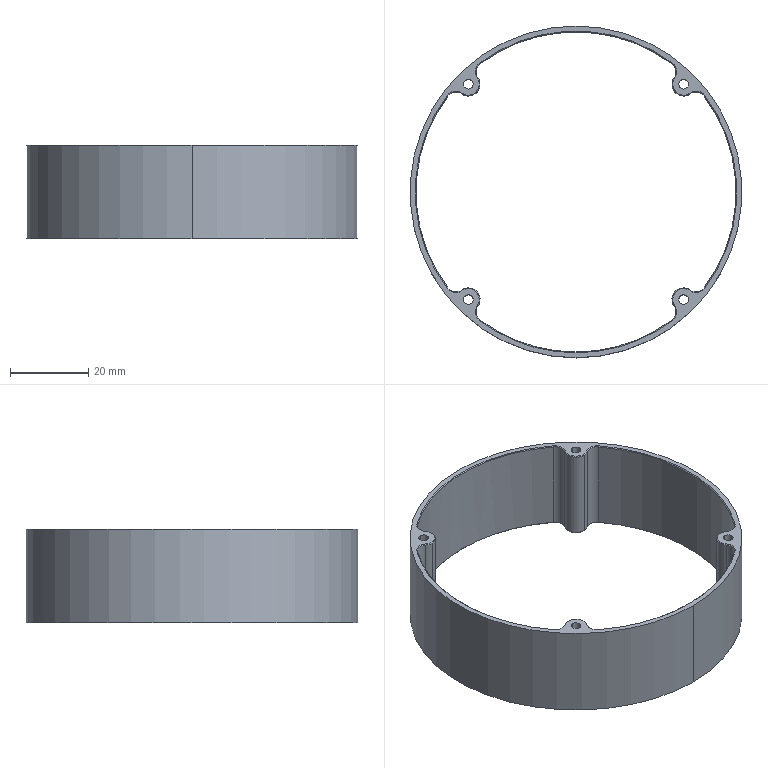NC program | NX | posted with a generic post | part box 85 x 85 x 24 mm
Lines 138 to 991 of 6793:
(PLANAR_MILL , TOOL : D10)
N250 T15 M6
N252 G54
N254 G17 G0 G90 X-2.703 Y-7.279 S9500 M3
N256 G43 Z30. H15
N258 Z1.
N260 G94 G1 X-2.578 Y-7.426 Z0.99 F1000.
N262 X-1.45 Y-8.911 Z0.892
N264 X-0.41 Y-10.46 Z0.794
N266 X0. Y-11.148 Z0.752
N268 X0.41 Y-10.46 Z0.71
N270 X1.45 Y-8.911 Z0.613
N272 X2.578 Y-7.426 Z0.515
N274 X3.79 Y-6.008 Z0.417
N276 X4.873 Y-4.873 Z0.335
N278 X6.008 Y-3.79 Z0.253
N280 X7.426 Y-2.578 Z0.155
N282 X8.911 Y-1.45 Z0.057
N284 X10.46 Y-0.41 Z-0.041
N286 X11.148 Y0. Z-0.083
N288 X10.46 Y0.41 Z-0.125
N290 X8.911 Y1.45 Z-0.222
N292 X7.426 Y2.578 Z-0.32
N294 X6.008 Y3.79 Z-0.418
N296 X4.879 Y4.879 Z-0.5
N298 X0.636 Y0.636
N300 G2 X0. Y1.288 R38.1 F2200.
N302 X-1.288 Y0. R38.1
N304 X0. Y-1.288 R38.1
N306 X1.288 Y0. R38.1
N308 X0.636 Y0.636 R38.1
N310 G1 X4.879 Y4.879
N312 G2 X0. Y11.148 R32.1
N314 X-11.148 Y0. R32.1
N316 X0. Y-11.148 R32.1
N318 X11.148 Y0. R32.1
N320 X4.879 Y4.879 R32.1
N322 G1 X9.122 Y9.122
N324 G2 X3.476 Y17.559 R26.1
N326 G3 X-3.476 Y17.559 R17.9
N328 G2 X-17.559 Y3.476 R26.1
N330 G3 X-17.559 Y-3.476 R17.9
N332 G2 X-3.476 Y-17.559 R26.1
N334 G3 X3.476 Y-17.559 R17.9
N336 G2 X17.559 Y-3.476 R26.1
N338 G3 X17.559 Y3.476 R17.9
N340 G2 X9.122 Y9.122 R26.1
N342 G1 X13.364 Y13.364
N344 G2 X8.136 Y22.472 R20.1
N346 G3 X-8.136 Y22.472 R23.9
N348 G2 X-22.472 Y8.136 R20.1
N350 G3 X-22.472 Y-8.136 R23.9
N352 G2 X-8.136 Y-22.472 R20.1
N354 G3 X8.136 Y-22.472 R23.9
N356 G2 X22.472 Y-8.136 R20.1
N358 G3 X22.472 Y8.136 R23.9
N360 G2 X13.364 Y13.364 R20.1
N362 G1 X17.607 Y17.607
N364 G2 X13.506 Y26.676 R14.1
N366 G3 X-13.506 Y26.676 R29.9
N368 G2 X-26.676 Y13.506 R14.1
N370 G3 X-26.676 Y-13.506 R29.9
N372 G2 X-13.506 Y-26.676 R14.1
N374 G3 X13.506 Y-26.676 R29.9
N376 G2 X26.676 Y-13.506 R14.1
N378 G3 X26.676 Y13.506 R29.9
N380 G2 X17.607 Y17.607 R14.1
N382 G1 X21.85 Y21.85
N384 G2 X19.826 Y29.929 R8.1
N386 G3 X-19.826 Y29.929 R35.9
N388 G2 X-29.929 Y19.826 R8.1
N390 G3 X-29.929 Y-19.826 R35.9
N392 G2 X-19.826 Y-29.929 R8.1
N394 G3 X19.826 Y-29.929 R35.9
N396 G2 X29.929 Y-19.826 R8.1
N398 G3 X29.929 Y19.826 R35.9
N400 G2 X21.85 Y21.85 R8.1
N402 G1 Z0.5
N404 G0 X-2.703 Y-7.279
N406 G1 X-2.578 Y-7.426 Z0.49 F1000.
N408 X-1.45 Y-8.911 Z0.392
N410 X-0.41 Y-10.46 Z0.294
N412 X0. Y-11.148 Z0.252
N414 X0.41 Y-10.46 Z0.21
N416 X1.45 Y-8.911 Z0.113
N418 X2.578 Y-7.426 Z0.015
N420 X3.79 Y-6.008 Z-0.083
N422 X4.873 Y-4.873 Z-0.165
N424 X6.008 Y-3.79 Z-0.247
N426 X7.426 Y-2.578 Z-0.345
N428 X8.911 Y-1.45 Z-0.443
N430 X10.46 Y-0.41 Z-0.541
N432 X11.148 Y0. Z-0.583
N434 X10.46 Y0.41 Z-0.625
N436 X8.911 Y1.45 Z-0.722
N438 X7.426 Y2.578 Z-0.82
N440 X6.008 Y3.79 Z-0.918
N442 X4.879 Y4.879 Z-1.
N444 X0.636 Y0.636
N446 G2 X0. Y1.288 R38.1 F2200.
N448 X-1.288 Y0. R38.1
N450 X0. Y-1.288 R38.1
N452 X1.288 Y0. R38.1
N454 X0.636 Y0.636 R38.1
N456 G1 X4.879 Y4.879
N458 G2 X0. Y11.148 R32.1
N460 X-11.148 Y0. R32.1
N462 X0. Y-11.148 R32.1
N464 X11.148 Y0. R32.1
N466 X4.879 Y4.879 R32.1
N468 G1 X9.122 Y9.122
N470 G2 X3.476 Y17.559 R26.1
N472 G3 X-3.476 Y17.559 R17.9
N474 G2 X-17.559 Y3.476 R26.1
N476 G3 X-17.559 Y-3.476 R17.9
N478 G2 X-3.476 Y-17.559 R26.1
N480 G3 X3.476 Y-17.559 R17.9
N482 G2 X17.559 Y-3.476 R26.1
N484 G3 X17.559 Y3.476 R17.9
N486 G2 X9.122 Y9.122 R26.1
N488 G1 X13.364 Y13.364
N490 G2 X8.136 Y22.472 R20.1
N492 G3 X-8.136 Y22.472 R23.9
N494 G2 X-22.472 Y8.136 R20.1
N496 G3 X-22.472 Y-8.136 R23.9
N498 G2 X-8.136 Y-22.472 R20.1
N500 G3 X8.136 Y-22.472 R23.9
N502 G2 X22.472 Y-8.136 R20.1
N504 G3 X22.472 Y8.136 R23.9
N506 G2 X13.364 Y13.364 R20.1
N508 G1 X17.607 Y17.607
N510 G2 X13.506 Y26.676 R14.1
N512 G3 X-13.506 Y26.676 R29.9
N514 G2 X-26.676 Y13.506 R14.1
N516 G3 X-26.676 Y-13.506 R29.9
N518 G2 X-13.506 Y-26.676 R14.1
N520 G3 X13.506 Y-26.676 R29.9
N522 G2 X26.676 Y-13.506 R14.1
N524 G3 X26.676 Y13.506 R29.9
N526 G2 X17.607 Y17.607 R14.1
N528 G1 X21.85 Y21.85
N530 G2 X19.826 Y29.929 R8.1
N532 G3 X-19.826 Y29.929 R35.9
N534 G2 X-29.929 Y19.826 R8.1
N536 G3 X-29.929 Y-19.826 R35.9
N538 G2 X-19.826 Y-29.929 R8.1
N540 G3 X19.826 Y-29.929 R35.9
N542 G2 X29.929 Y-19.826 R8.1
N544 G3 X29.929 Y19.826 R35.9
N546 G2 X21.85 Y21.85 R8.1
N548 G1 Z0.
N550 G0 X-2.703 Y-7.279
N552 G1 X-2.578 Y-7.426 Z-0.01 F1000.
N554 X-1.45 Y-8.911 Z-0.108
N556 X-0.41 Y-10.46 Z-0.206
N558 X0. Y-11.148 Z-0.248
N560 X0.41 Y-10.46 Z-0.29
N562 X1.45 Y-8.911 Z-0.387
N564 X2.578 Y-7.426 Z-0.485
N566 X3.79 Y-6.008 Z-0.583
N568 X4.873 Y-4.873 Z-0.665
N570 X6.008 Y-3.79 Z-0.747
N572 X7.426 Y-2.578 Z-0.845
N574 X8.911 Y-1.45 Z-0.943
N576 X10.46 Y-0.41 Z-1.041
N578 X11.148 Y0. Z-1.083
N580 X10.46 Y0.41 Z-1.125
N582 X8.911 Y1.45 Z-1.222
N584 X7.426 Y2.578 Z-1.32
N586 X6.008 Y3.79 Z-1.418
N588 X4.879 Y4.879 Z-1.5
N590 X0.636 Y0.636
N592 G2 X0. Y1.288 R38.1 F2200.
N594 X-1.288 Y0. R38.1
N596 X0. Y-1.288 R38.1
N598 X1.288 Y0. R38.1
N600 X0.636 Y0.636 R38.1
N602 G1 X4.879 Y4.879
N604 G2 X0. Y11.148 R32.1
N606 X-11.148 Y0. R32.1
N608 X0. Y-11.148 R32.1
N610 X11.148 Y0. R32.1
N612 X4.879 Y4.879 R32.1
N614 G1 X9.122 Y9.122
N616 G2 X3.476 Y17.559 R26.1
N618 G3 X-3.476 Y17.559 R17.9
N620 G2 X-17.559 Y3.476 R26.1
N622 G3 X-17.559 Y-3.476 R17.9
N624 G2 X-3.476 Y-17.559 R26.1
N626 G3 X3.476 Y-17.559 R17.9
N628 G2 X17.559 Y-3.476 R26.1
N630 G3 X17.559 Y3.476 R17.9
N632 G2 X9.122 Y9.122 R26.1
N634 G1 X13.364 Y13.364
N636 G2 X8.136 Y22.472 R20.1
N638 G3 X-8.136 Y22.472 R23.9
N640 G2 X-22.472 Y8.136 R20.1
N642 G3 X-22.472 Y-8.136 R23.9
N644 G2 X-8.136 Y-22.472 R20.1
N646 G3 X8.136 Y-22.472 R23.9
N648 G2 X22.472 Y-8.136 R20.1
N650 G3 X22.472 Y8.136 R23.9
N652 G2 X13.364 Y13.364 R20.1
N654 G1 X17.607 Y17.607
N656 G2 X13.506 Y26.676 R14.1
N658 G3 X-13.506 Y26.676 R29.9
N660 G2 X-26.676 Y13.506 R14.1
N662 G3 X-26.676 Y-13.506 R29.9
N664 G2 X-13.506 Y-26.676 R14.1
N666 G3 X13.506 Y-26.676 R29.9
N668 G2 X26.676 Y-13.506 R14.1
N670 G3 X26.676 Y13.506 R29.9
N672 G2 X17.607 Y17.607 R14.1
N674 G1 X21.85 Y21.85
N676 G2 X19.826 Y29.929 R8.1
N678 G3 X-19.826 Y29.929 R35.9
N680 G2 X-29.929 Y19.826 R8.1
N682 G3 X-29.929 Y-19.826 R35.9
N684 G2 X-19.826 Y-29.929 R8.1
N686 G3 X19.826 Y-29.929 R35.9
N688 G2 X29.929 Y-19.826 R8.1
N690 G3 X29.929 Y19.826 R35.9
N692 G2 X21.85 Y21.85 R8.1
N694 G1 Z-0.5
N696 G0 X-2.703 Y-7.279
N698 G1 X-2.578 Y-7.426 Z-0.51 F1000.
N700 X-1.45 Y-8.911 Z-0.608
N702 X-0.41 Y-10.46 Z-0.706
N704 X0. Y-11.148 Z-0.748
N706 X0.41 Y-10.46 Z-0.79
N708 X1.45 Y-8.911 Z-0.887
N710 X2.578 Y-7.426 Z-0.985
N712 X3.79 Y-6.008 Z-1.083
N714 X4.873 Y-4.873 Z-1.165
N716 X6.008 Y-3.79 Z-1.247
N718 X7.426 Y-2.578 Z-1.345
N720 X8.911 Y-1.45 Z-1.443
N722 X10.46 Y-0.41 Z-1.541
N724 X11.148 Y0. Z-1.583
N726 X10.46 Y0.41 Z-1.625
N728 X8.911 Y1.45 Z-1.722
N730 X7.426 Y2.578 Z-1.82
N732 X6.008 Y3.79 Z-1.918
N734 X4.879 Y4.879 Z-2.
N736 X0.636 Y0.636
N738 G2 X0. Y1.288 R38.1 F2200.
N740 X-1.288 Y0. R38.1
N742 X0. Y-1.288 R38.1
N744 X1.288 Y0. R38.1
N746 X0.636 Y0.636 R38.1
N748 G1 X4.879 Y4.879
N750 G2 X0. Y11.148 R32.1
N752 X-11.148 Y0. R32.1
N754 X0. Y-11.148 R32.1
N756 X11.148 Y0. R32.1
N758 X4.879 Y4.879 R32.1
N760 G1 X9.122 Y9.122
N762 G2 X3.476 Y17.559 R26.1
N764 G3 X-3.476 Y17.559 R17.9
N766 G2 X-17.559 Y3.476 R26.1
N768 G3 X-17.559 Y-3.476 R17.9
N770 G2 X-3.476 Y-17.559 R26.1
N772 G3 X3.476 Y-17.559 R17.9
N774 G2 X17.559 Y-3.476 R26.1
N776 G3 X17.559 Y3.476 R17.9
N778 G2 X9.122 Y9.122 R26.1
N780 G1 X13.364 Y13.364
N782 G2 X8.136 Y22.472 R20.1
N784 G3 X-8.136 Y22.472 R23.9
N786 G2 X-22.472 Y8.136 R20.1
N788 G3 X-22.472 Y-8.136 R23.9
N790 G2 X-8.136 Y-22.472 R20.1
N792 G3 X8.136 Y-22.472 R23.9
N794 G2 X22.472 Y-8.136 R20.1
N796 G3 X22.472 Y8.136 R23.9
N798 G2 X13.364 Y13.364 R20.1
N800 G1 X17.607 Y17.607
N802 G2 X13.506 Y26.676 R14.1
N804 G3 X-13.506 Y26.676 R29.9
N806 G2 X-26.676 Y13.506 R14.1
N808 G3 X-26.676 Y-13.506 R29.9
N810 G2 X-13.506 Y-26.676 R14.1
N812 G3 X13.506 Y-26.676 R29.9
N814 G2 X26.676 Y-13.506 R14.1
N816 G3 X26.676 Y13.506 R29.9
N818 G2 X17.607 Y17.607 R14.1
N820 G1 X21.85 Y21.85
N822 G2 X19.826 Y29.929 R8.1
N824 G3 X-19.826 Y29.929 R35.9
N826 G2 X-29.929 Y19.826 R8.1
N828 G3 X-29.929 Y-19.826 R35.9
N830 G2 X-19.826 Y-29.929 R8.1
N832 G3 X19.826 Y-29.929 R35.9
N834 G2 X29.929 Y-19.826 R8.1
N836 G3 X29.929 Y19.826 R35.9
N838 G2 X21.85 Y21.85 R8.1
N840 G1 Z-1.
N842 G0 X-2.703 Y-7.279
N844 G1 X-2.578 Y-7.426 Z-1.01 F1000.
N846 X-1.45 Y-8.911 Z-1.108
N848 X-0.41 Y-10.46 Z-1.206
N850 X0. Y-11.148 Z-1.248
N852 X0.41 Y-10.46 Z-1.29
N854 X1.45 Y-8.911 Z-1.387
N856 X2.578 Y-7.426 Z-1.485
N858 X3.79 Y-6.008 Z-1.583
N860 X4.873 Y-4.873 Z-1.665
N862 X6.008 Y-3.79 Z-1.747
N864 X7.426 Y-2.578 Z-1.845
N866 X8.911 Y-1.45 Z-1.943
N868 X10.46 Y-0.41 Z-2.041
N870 X11.148 Y0. Z-2.083
N872 X10.46 Y0.41 Z-2.125
N874 X8.911 Y1.45 Z-2.222
N876 X7.426 Y2.578 Z-2.32
N878 X6.008 Y3.79 Z-2.418
N880 X4.879 Y4.879 Z-2.5
N882 X0.636 Y0.636
N884 G2 X0. Y1.288 R38.1 F2200.
N886 X-1.288 Y0. R38.1
N888 X0. Y-1.288 R38.1
N890 X1.288 Y0. R38.1
N892 X0.636 Y0.636 R38.1
N894 G1 X4.879 Y4.879
N896 G2 X0. Y11.148 R32.1
N898 X-11.148 Y0. R32.1
N900 X0. Y-11.148 R32.1
N902 X11.148 Y0. R32.1
N904 X4.879 Y4.879 R32.1
N906 G1 X9.122 Y9.122
N908 G2 X3.476 Y17.559 R26.1
N910 G3 X-3.476 Y17.559 R17.9
N912 G2 X-17.559 Y3.476 R26.1
N914 G3 X-17.559 Y-3.476 R17.9
N916 G2 X-3.476 Y-17.559 R26.1
N918 G3 X3.476 Y-17.559 R17.9
N920 G2 X17.559 Y-3.476 R26.1
N922 G3 X17.559 Y3.476 R17.9
N924 G2 X9.122 Y9.122 R26.1
N926 G1 X13.364 Y13.364
N928 G2 X8.136 Y22.472 R20.1
N930 G3 X-8.136 Y22.472 R23.9
N932 G2 X-22.472 Y8.136 R20.1
N934 G3 X-22.472 Y-8.136 R23.9
N936 G2 X-8.136 Y-22.472 R20.1
N938 G3 X8.136 Y-22.472 R23.9
N940 G2 X22.472 Y-8.136 R20.1
N942 G3 X22.472 Y8.136 R23.9
N944 G2 X13.364 Y13.364 R20.1
N946 G1 X17.607 Y17.607
N948 G2 X13.506 Y26.676 R14.1
N950 G3 X-13.506 Y26.676 R29.9
N952 G2 X-26.676 Y13.506 R14.1
N954 G3 X-26.676 Y-13.506 R29.9
N956 G2 X-13.506 Y-26.676 R14.1
N958 G3 X13.506 Y-26.676 R29.9
N960 G2 X26.676 Y-13.506 R14.1
N962 G3 X26.676 Y13.506 R29.9
N964 G2 X17.607 Y17.607 R14.1
N966 G1 X21.85 Y21.85
N968 G2 X19.826 Y29.929 R8.1
N970 G3 X-19.826 Y29.929 R35.9
N972 G2 X-29.929 Y19.826 R8.1
N974 G3 X-29.929 Y-19.826 R35.9
N976 G2 X-19.826 Y-29.929 R8.1
N978 G3 X19.826 Y-29.929 R35.9
N980 G2 X29.929 Y-19.826 R8.1
N982 G3 X29.929 Y19.826 R35.9
N984 G2 X21.85 Y21.85 R8.1
N986 G1 Z-1.5
N988 G0 X-2.703 Y-7.279
N990 G1 X-2.578 Y-7.426 Z-1.51 F1000.
N992 X-1.45 Y-8.911 Z-1.608
N994 X-0.41 Y-10.46 Z-1.706
N996 X0. Y-11.148 Z-1.748
N998 X0.41 Y-10.46 Z-1.79
N1000 X1.45 Y-8.911 Z-1.887
N1002 X2.578 Y-7.426 Z-1.985
N1004 X3.79 Y-6.008 Z-2.083
N1006 X4.873 Y-4.873 Z-2.165
N1008 X6.008 Y-3.79 Z-2.247
N1010 X7.426 Y-2.578 Z-2.345
N1012 X8.911 Y-1.45 Z-2.443
N1014 X10.46 Y-0.41 Z-2.541
N1016 X11.148 Y0. Z-2.583
N1018 X10.46 Y0.41 Z-2.625
N1020 X8.911 Y1.45 Z-2.722
N1022 X7.426 Y2.578 Z-2.82
N1024 X6.008 Y3.79 Z-2.918
N1026 X4.879 Y4.879 Z-3.
N1028 X0.636 Y0.636
N1030 G2 X0. Y1.288 R38.1 F2200.
N1032 X-1.288 Y0. R38.1
N1034 X0. Y-1.288 R38.1
N1036 X1.288 Y0. R38.1
N1038 X0.636 Y0.636 R38.1
N1040 G1 X4.879 Y4.879
N1042 G2 X0. Y11.148 R32.1
N1044 X-11.148 Y0. R32.1
N1046 X0. Y-11.148 R32.1
N1048 X11.148 Y0. R32.1
N1050 X4.879 Y4.879 R32.1
N1052 G1 X9.122 Y9.122
N1054 G2 X3.476 Y17.559 R26.1
N1056 G3 X-3.476 Y17.559 R17.9
N1058 G2 X-17.559 Y3.476 R26.1
N1060 G3 X-17.559 Y-3.476 R17.9
N1062 G2 X-3.476 Y-17.559 R26.1
N1064 G3 X3.476 Y-17.559 R17.9
N1066 G2 X17.559 Y-3.476 R26.1
N1068 G3 X17.559 Y3.476 R17.9
N1070 G2 X9.122 Y9.122 R26.1
N1072 G1 X13.364 Y13.364
N1074 G2 X8.136 Y22.472 R20.1
N1076 G3 X-8.136 Y22.472 R23.9
N1078 G2 X-22.472 Y8.136 R20.1
N1080 G3 X-22.472 Y-8.136 R23.9
N1082 G2 X-8.136 Y-22.472 R20.1
N1084 G3 X8.136 Y-22.472 R23.9
N1086 G2 X22.472 Y-8.136 R20.1
N1088 G3 X22.472 Y8.136 R23.9
N1090 G2 X13.364 Y13.364 R20.1
N1092 G1 X17.607 Y17.607
N1094 G2 X13.506 Y26.676 R14.1
N1096 G3 X-13.506 Y26.676 R29.9
N1098 G2 X-26.676 Y13.506 R14.1
N1100 G3 X-26.676 Y-13.506 R29.9
N1102 G2 X-13.506 Y-26.676 R14.1
N1104 G3 X13.506 Y-26.676 R29.9
N1106 G2 X26.676 Y-13.506 R14.1
N1108 G3 X26.676 Y13.506 R29.9
N1110 G2 X17.607 Y17.607 R14.1
N1112 G1 X21.85 Y21.85
N1114 G2 X19.826 Y29.929 R8.1
N1116 G3 X-19.826 Y29.929 R35.9
N1118 G2 X-29.929 Y19.826 R8.1
N1120 G3 X-29.929 Y-19.826 R35.9
N1122 G2 X-19.826 Y-29.929 R8.1
N1124 G3 X19.826 Y-29.929 R35.9
N1126 G2 X29.929 Y-19.826 R8.1
N1128 G3 X29.929 Y19.826 R35.9
N1130 G2 X21.85 Y21.85 R8.1
N1132 G1 Z-2.
N1134 G0 X-2.703 Y-7.279
N1136 G1 X-2.578 Y-7.426 Z-2.01 F1000.
N1138 X-1.45 Y-8.911 Z-2.108
N1140 X-0.41 Y-10.46 Z-2.206
N1142 X0. Y-11.148 Z-2.248
N1144 X0.41 Y-10.46 Z-2.29
N1146 X1.45 Y-8.911 Z-2.387
N1148 X2.578 Y-7.426 Z-2.485
N1150 X3.79 Y-6.008 Z-2.583
N1152 X4.873 Y-4.873 Z-2.665
N1154 X6.008 Y-3.79 Z-2.747
N1156 X7.426 Y-2.578 Z-2.845
N1158 X8.911 Y-1.45 Z-2.943
N1160 X10.46 Y-0.41 Z-3.041
N1162 X11.148 Y0. Z-3.083
N1164 X10.46 Y0.41 Z-3.125
N1166 X8.911 Y1.45 Z-3.222
N1168 X7.426 Y2.578 Z-3.32
N1170 X6.008 Y3.79 Z-3.418
N1172 X4.879 Y4.879 Z-3.5
N1174 X0.636 Y0.636
N1176 G2 X0. Y1.288 R38.1 F2200.
N1178 X-1.288 Y0. R38.1
N1180 X0. Y-1.288 R38.1
N1182 X1.288 Y0. R38.1
N1184 X0.636 Y0.636 R38.1
N1186 G1 X4.879 Y4.879
N1188 G2 X0. Y11.148 R32.1
N1190 X-11.148 Y0. R32.1
N1192 X0. Y-11.148 R32.1
N1194 X11.148 Y0. R32.1
N1196 X4.879 Y4.879 R32.1
N1198 G1 X9.122 Y9.122
N1200 G2 X3.476 Y17.559 R26.1
N1202 G3 X-3.476 Y17.559 R17.9
N1204 G2 X-17.559 Y3.476 R26.1
N1206 G3 X-17.559 Y-3.476 R17.9
N1208 G2 X-3.476 Y-17.559 R26.1
N1210 G3 X3.476 Y-17.559 R17.9
N1212 G2 X17.559 Y-3.476 R26.1
N1214 G3 X17.559 Y3.476 R17.9
N1216 G2 X9.122 Y9.122 R26.1
N1218 G1 X13.364 Y13.364
N1220 G2 X8.136 Y22.472 R20.1
N1222 G3 X-8.136 Y22.472 R23.9
N1224 G2 X-22.472 Y8.136 R20.1
N1226 G3 X-22.472 Y-8.136 R23.9
N1228 G2 X-8.136 Y-22.472 R20.1
N1230 G3 X8.136 Y-22.472 R23.9
N1232 G2 X22.472 Y-8.136 R20.1
N1234 G3 X22.472 Y8.136 R23.9
N1236 G2 X13.364 Y13.364 R20.1
N1238 G1 X17.607 Y17.607
N1240 G2 X13.506 Y26.676 R14.1
N1242 G3 X-13.506 Y26.676 R29.9
N1244 G2 X-26.676 Y13.506 R14.1
N1246 G3 X-26.676 Y-13.506 R29.9
N1248 G2 X-13.506 Y-26.676 R14.1
N1250 G3 X13.506 Y-26.676 R29.9
N1252 G2 X26.676 Y-13.506 R14.1
N1254 G3 X26.676 Y13.506 R29.9
N1256 G2 X17.607 Y17.607 R14.1
N1258 G1 X21.85 Y21.85
N1260 G2 X19.826 Y29.929 R8.1
N1262 G3 X-19.826 Y29.929 R35.9
N1264 G2 X-29.929 Y19.826 R8.1
N1266 G3 X-29.929 Y-19.826 R35.9
N1268 G2 X-19.826 Y-29.929 R8.1
N1270 G3 X19.826 Y-29.929 R35.9
N1272 G2 X29.929 Y-19.826 R8.1
N1274 G3 X29.929 Y19.826 R35.9
N1276 G2 X21.85 Y21.85 R8.1
N1278 G1 Z-2.5
N1280 G0 X-2.703 Y-7.279
N1282 G1 X-2.578 Y-7.426 Z-2.51 F1000.
N1284 X-1.45 Y-8.911 Z-2.608
N1286 X-0.41 Y-10.46 Z-2.706
N1288 X0. Y-11.148 Z-2.748
N1290 X0.41 Y-10.46 Z-2.79
N1292 X1.45 Y-8.911 Z-2.887
N1294 X2.578 Y-7.426 Z-2.985
N1296 X3.79 Y-6.008 Z-3.083
N1298 X4.873 Y-4.873 Z-3.165
N1300 X6.008 Y-3.79 Z-3.247
N1302 X7.426 Y-2.578 Z-3.345
N1304 X8.911 Y-1.45 Z-3.443
N1306 X10.46 Y-0.41 Z-3.541
N1308 X11.148 Y0. Z-3.583
N1310 X10.46 Y0.41 Z-3.625
N1312 X8.911 Y1.45 Z-3.722
N1314 X7.426 Y2.578 Z-3.82
N1316 X6.008 Y3.79 Z-3.918
N1318 X4.879 Y4.879 Z-4.
N1320 X0.636 Y0.636
N1322 G2 X0. Y1.288 R38.1 F2200.
N1324 X-1.288 Y0. R38.1
N1326 X0. Y-1.288 R38.1
N1328 X1.288 Y0. R38.1
N1330 X0.636 Y0.636 R38.1
N1332 G1 X4.879 Y4.879
N1334 G2 X0. Y11.148 R32.1
N1336 X-11.148 Y0. R32.1
N1338 X0. Y-11.148 R32.1
N1340 X11.148 Y0. R32.1
N1342 X4.879 Y4.879 R32.1
N1344 G1 X9.122 Y9.122
N1346 G2 X3.476 Y17.559 R26.1
N1348 G3 X-3.476 Y17.559 R17.9
N1350 G2 X-17.559 Y3.476 R26.1
N1352 G3 X-17.559 Y-3.476 R17.9
N1354 G2 X-3.476 Y-17.559 R26.1
N1356 G3 X3.476 Y-17.559 R17.9
N1358 G2 X17.559 Y-3.476 R26.1
N1360 G3 X17.559 Y3.476 R17.9
N1362 G2 X9.122 Y9.122 R26.1
N1364 G1 X13.364 Y13.364
N1366 G2 X8.136 Y22.472 R20.1
N1368 G3 X-8.136 Y22.472 R23.9
N1370 G2 X-22.472 Y8.136 R20.1
N1372 G3 X-22.472 Y-8.136 R23.9
N1374 G2 X-8.136 Y-22.472 R20.1
N1376 G3 X8.136 Y-22.472 R23.9
N1378 G2 X22.472 Y-8.136 R20.1
N1380 G3 X22.472 Y8.136 R23.9
N1382 G2 X13.364 Y13.364 R20.1
N1384 G1 X17.607 Y17.607
N1386 G2 X13.506 Y26.676 R14.1
N1388 G3 X-13.506 Y26.676 R29.9
N1390 G2 X-26.676 Y13.506 R14.1
N1392 G3 X-26.676 Y-13.506 R29.9
N1394 G2 X-13.506 Y-26.676 R14.1
N1396 G3 X13.506 Y-26.676 R29.9
N1398 G2 X26.676 Y-13.506 R14.1
N1400 G3 X26.676 Y13.506 R29.9
N1402 G2 X17.607 Y17.607 R14.1
N1404 G1 X21.85 Y21.85
N1406 G2 X19.826 Y29.929 R8.1
N1408 G3 X-19.826 Y29.929 R35.9
N1410 G2 X-29.929 Y19.826 R8.1
N1412 G3 X-29.929 Y-19.826 R35.9
N1414 G2 X-19.826 Y-29.929 R8.1
N1416 G3 X19.826 Y-29.929 R35.9
N1418 G2 X29.929 Y-19.826 R8.1
N1420 G3 X29.929 Y19.826 R35.9
N1422 G2 X21.85 Y21.85 R8.1
N1424 G1 Z-3.
N1426 G0 X-2.703 Y-7.279
N1428 G1 X-2.578 Y-7.426 Z-3.01 F1000.
N1430 X-1.45 Y-8.911 Z-3.108
N1432 X-0.41 Y-10.46 Z-3.206
N1434 X0. Y-11.148 Z-3.248
N1436 X0.41 Y-10.46 Z-3.29
N1438 X1.45 Y-8.911 Z-3.387
N1440 X2.578 Y-7.426 Z-3.485
N1442 X3.79 Y-6.008 Z-3.583
N1444 X4.873 Y-4.873 Z-3.665
N1446 X6.008 Y-3.79 Z-3.747
N1448 X7.426 Y-2.578 Z-3.845
N1450 X8.911 Y-1.45 Z-3.943
N1452 X10.46 Y-0.41 Z-4.041
N1454 X11.148 Y0. Z-4.083
N1456 X10.46 Y0.41 Z-4.125
N1458 X8.911 Y1.45 Z-4.222
N1460 X7.426 Y2.578 Z-4.32
N1462 X6.008 Y3.79 Z-4.418
N1464 X4.879 Y4.879 Z-4.5
N1466 X0.636 Y0.636
N1468 G2 X0. Y1.288 R38.1 F2200.
N1470 X-1.288 Y0. R38.1
N1472 X0. Y-1.288 R38.1
N1474 X1.288 Y0. R38.1
N1476 X0.636 Y0.636 R38.1
N1478 G1 X4.879 Y4.879
N1480 G2 X0. Y11.148 R32.1
N1482 X-11.148 Y0. R32.1
N1484 X0. Y-11.148 R32.1
N1486 X11.148 Y0. R32.1
N1488 X4.879 Y4.879 R32.1
N1490 G1 X9.122 Y9.122
N1492 G2 X3.476 Y17.559 R26.1
N1494 G3 X-3.476 Y17.559 R17.9
N1496 G2 X-17.559 Y3.476 R26.1
N1498 G3 X-17.559 Y-3.476 R17.9
N1500 G2 X-3.476 Y-17.559 R26.1
N1502 G3 X3.476 Y-17.559 R17.9
N1504 G2 X17.559 Y-3.476 R26.1
N1506 G3 X17.559 Y3.476 R17.9
N1508 G2 X9.122 Y9.122 R26.1
N1510 G1 X13.364 Y13.364
N1512 G2 X8.136 Y22.472 R20.1
N1514 G3 X-8.136 Y22.472 R23.9
N1516 G2 X-22.472 Y8.136 R20.1
N1518 G3 X-22.472 Y-8.136 R23.9
N1520 G2 X-8.136 Y-22.472 R20.1
N1522 G3 X8.136 Y-22.472 R23.9
N1524 G2 X22.472 Y-8.136 R20.1
N1526 G3 X22.472 Y8.136 R23.9
N1528 G2 X13.364 Y13.364 R20.1
N1530 G1 X17.607 Y17.607
N1532 G2 X13.506 Y26.676 R14.1
N1534 G3 X-13.506 Y26.676 R29.9
N1536 G2 X-26.676 Y13.506 R14.1
N1538 G3 X-26.676 Y-13.506 R29.9
N1540 G2 X-13.506 Y-26.676 R14.1
N1542 G3 X13.506 Y-26.676 R29.9
N1544 G2 X26.676 Y-13.506 R14.1
N1546 G3 X26.676 Y13.506 R29.9
N1548 G2 X17.607 Y17.607 R14.1
N1550 G1 X21.85 Y21.85
N1552 G2 X19.826 Y29.929 R8.1
N1554 G3 X-19.826 Y29.929 R35.9
N1556 G2 X-29.929 Y19.826 R8.1
N1558 G3 X-29.929 Y-19.826 R35.9
N1560 G2 X-19.826 Y-29.929 R8.1
N1562 G3 X19.826 Y-29.929 R35.9
N1564 G2 X29.929 Y-19.826 R8.1
N1566 G3 X29.929 Y19.826 R35.9
N1568 G2 X21.85 Y21.85 R8.1
N1570 G1 Z-3.5
N1572 G0 X-2.703 Y-7.279
N1574 G1 X-2.578 Y-7.426 Z-3.51 F1000.
N1576 X-1.45 Y-8.911 Z-3.608
N1578 X-0.41 Y-10.46 Z-3.706
N1580 X0. Y-11.148 Z-3.748
N1582 X0.41 Y-10.46 Z-3.79
N1584 X1.45 Y-8.911 Z-3.887
N1586 X2.578 Y-7.426 Z-3.985
N1588 X3.79 Y-6.008 Z-4.083
N1590 X4.873 Y-4.873 Z-4.165
N1592 X6.008 Y-3.79 Z-4.247
N1594 X7.426 Y-2.578 Z-4.345
N1596 X8.911 Y-1.45 Z-4.443
N1598 X10.46 Y-0.41 Z-4.541
N1600 X11.148 Y0. Z-4.583
N1602 X10.46 Y0.41 Z-4.625
N1604 X8.911 Y1.45 Z-4.722
N1606 X7.426 Y2.578 Z-4.82
N1608 X6.008 Y3.79 Z-4.918
N1610 X4.879 Y4.879 Z-5.
N1612 X0.636 Y0.636
N1614 G2 X0. Y1.288 R38.1 F2200.
N1616 X-1.288 Y0. R38.1
N1618 X0. Y-1.288 R38.1
N1620 X1.288 Y0. R38.1
N1622 X0.636 Y0.636 R38.1
N1624 G1 X4.879 Y4.879
N1626 G2 X0. Y11.148 R32.1
N1628 X-11.148 Y0. R32.1
N1630 X0. Y-11.148 R32.1
N1632 X11.148 Y0. R32.1
N1634 X4.879 Y4.879 R32.1
N1636 G1 X9.122 Y9.122
N1638 G2 X3.476 Y17.559 R26.1
N1640 G3 X-3.476 Y17.559 R17.9
N1642 G2 X-17.559 Y3.476 R26.1
N1644 G3 X-17.559 Y-3.476 R17.9
N1646 G2 X-3.476 Y-17.559 R26.1
N1648 G3 X3.476 Y-17.559 R17.9
N1650 G2 X17.559 Y-3.476 R26.1
N1652 G3 X17.559 Y3.476 R17.9
N1654 G2 X9.122 Y9.122 R26.1
N1656 G1 X13.364 Y13.364
N1658 G2 X8.136 Y22.472 R20.1
N1660 G3 X-8.136 Y22.472 R23.9
N1662 G2 X-22.472 Y8.136 R20.1
N1664 G3 X-22.472 Y-8.136 R23.9
N1666 G2 X-8.136 Y-22.472 R20.1
N1668 G3 X8.136 Y-22.472 R23.9
N1670 G2 X22.472 Y-8.136 R20.1
N1672 G3 X22.472 Y8.136 R23.9
N1674 G2 X13.364 Y13.364 R20.1
N1676 G1 X17.607 Y17.607
N1678 G2 X13.506 Y26.676 R14.1
N1680 G3 X-13.506 Y26.676 R29.9
N1682 G2 X-26.676 Y13.506 R14.1
N1684 G3 X-26.676 Y-13.506 R29.9
N1686 G2 X-13.506 Y-26.676 R14.1
N1688 G3 X13.506 Y-26.676 R29.9
N1690 G2 X26.676 Y-13.506 R14.1
N1692 G3 X26.676 Y13.506 R29.9
N1694 G2 X17.607 Y17.607 R14.1
N1696 G1 X21.85 Y21.85
N1698 G2 X19.826 Y29.929 R8.1
N1700 G3 X-19.826 Y29.929 R35.9
N1702 G2 X-29.929 Y19.826 R8.1
N1704 G3 X-29.929 Y-19.826 R35.9
N1706 G2 X-19.826 Y-29.929 R8.1
N1708 G3 X19.826 Y-29.929 R35.9
N1710 G2 X29.929 Y-19.826 R8.1
N1712 G3 X29.929 Y19.826 R35.9
N1714 G2 X21.85 Y21.85 R8.1
N1716 G1 Z-4.
N1718 G0 X-2.703 Y-7.279
N1720 G1 X-2.578 Y-7.426 Z-4.01 F1000.
N1722 X-1.45 Y-8.911 Z-4.108
N1724 X-0.41 Y-10.46 Z-4.206
N1726 X0. Y-11.148 Z-4.248
N1728 X0.41 Y-10.46 Z-4.29
N1730 X1.45 Y-8.911 Z-4.387
N1732 X2.578 Y-7.426 Z-4.485
N1734 X3.79 Y-6.008 Z-4.583
N1736 X4.873 Y-4.873 Z-4.665
N1738 X6.008 Y-3.79 Z-4.747
N1740 X7.426 Y-2.578 Z-4.845
N1742 X8.911 Y-1.45 Z-4.943
N1744 X10.46 Y-0.41 Z-5.041
N1746 X11.148 Y0. Z-5.083
N1748 X10.46 Y0.41 Z-5.125
N1750 X8.911 Y1.45 Z-5.222
N1752 X7.426 Y2.578 Z-5.32
N1754 X6.008 Y3.79 Z-5.418
N1756 X4.879 Y4.879 Z-5.5
N1758 X0.636 Y0.636
N1760 G2 X0. Y1.288 R38.1 F2200.
N1762 X-1.288 Y0. R38.1
N1764 X0. Y-1.288 R38.1
N1766 X1.288 Y0. R38.1
N1768 X0.636 Y0.636 R38.1
N1770 G1 X4.879 Y4.879
N1772 G2 X0. Y11.148 R32.1
N1774 X-11.148 Y0. R32.1
N1776 X0. Y-11.148 R32.1
N1778 X11.148 Y0. R32.1
N1780 X4.879 Y4.879 R32.1
N1782 G1 X9.122 Y9.122
N1784 G2 X3.476 Y17.559 R26.1
N1786 G3 X-3.476 Y17.559 R17.9
N1788 G2 X-17.559 Y3.476 R26.1
N1790 G3 X-17.559 Y-3.476 R17.9
N1792 G2 X-3.476 Y-17.559 R26.1
N1794 G3 X3.476 Y-17.559 R17.9
N1796 G2 X17.559 Y-3.476 R26.1
N1798 G3 X17.559 Y3.476 R17.9
N1800 G2 X9.122 Y9.122 R26.1
N1802 G1 X13.364 Y13.364
N1804 G2 X8.136 Y22.472 R20.1
N1806 G3 X-8.136 Y22.472 R23.9
N1808 G2 X-22.472 Y8.136 R20.1
N1810 G3 X-22.472 Y-8.136 R23.9
N1812 G2 X-8.136 Y-22.472 R20.1
N1814 G3 X8.136 Y-22.472 R23.9
N1816 G2 X22.472 Y-8.136 R20.1
N1818 G3 X22.472 Y8.136 R23.9
N1820 G2 X13.364 Y13.364 R20.1
N1822 G1 X17.607 Y17.607
N1824 G2 X13.506 Y26.676 R14.1
N1826 G3 X-13.506 Y26.676 R29.9
N1828 G2 X-26.676 Y13.506 R14.1
N1830 G3 X-26.676 Y-13.506 R29.9
N1832 G2 X-13.506 Y-26.676 R14.1
N1834 G3 X13.506 Y-26.676 R29.9
N1836 G2 X26.676 Y-13.506 R14.1
N1838 G3 X26.676 Y13.506 R29.9
N1840 G2 X17.607 Y17.607 R14.1
N1842 G1 X21.85 Y21.85
N1844 G2 X19.826 Y29.929 R8.1
N1846 G3 X-19.826 Y29.929 R35.9
N1848 G2 X-29.929 Y19.826 R8.1
N1850 G3 X-29.929 Y-19.826 R35.9
N1852 G2 X-19.826 Y-29.929 R8.1
N1854 G3 X19.826 Y-29.929 R35.9
N1856 G2 X29.929 Y-19.826 R8.1
N1858 G3 X29.929 Y19.826 R35.9
N1860 G2 X21.85 Y21.85 R8.1
N1862 G1 Z-4.5
N1864 G0 X-2.703 Y-7.279
N1866 G1 X-2.578 Y-7.426 Z-4.51 F1000.
N1868 X-1.45 Y-8.911 Z-4.608
N1870 X-0.41 Y-10.46 Z-4.706
N1872 X0. Y-11.148 Z-4.748
N1874 X0.41 Y-10.46 Z-4.79
N1876 X1.45 Y-8.911 Z-4.887
N1878 X2.578 Y-7.426 Z-4.985
N1880 X3.79 Y-6.008 Z-5.083
N1882 X4.873 Y-4.873 Z-5.165
N1884 X6.008 Y-3.79 Z-5.247
N1886 X7.426 Y-2.578 Z-5.345
N1888 X8.911 Y-1.45 Z-5.443
N1890 X10.46 Y-0.41 Z-5.541
N1892 X11.148 Y0. Z-5.583
N1894 X10.46 Y0.41 Z-5.625
N1896 X8.911 Y1.45 Z-5.722
N1898 X7.426 Y2.578 Z-5.82
N1900 X6.008 Y3.79 Z-5.918
N1902 X4.879 Y4.879 Z-6.
N1904 X0.636 Y0.636
N1906 G2 X0. Y1.288 R38.1 F2200.
N1908 X-1.288 Y0. R38.1
N1910 X0. Y-1.288 R38.1
N1912 X1.288 Y0. R38.1
N1914 X0.636 Y0.636 R38.1
N1916 G1 X4.879 Y4.879
N1918 G2 X0. Y11.148 R32.1
N1920 X-11.148 Y0. R32.1
N1922 X0. Y-11.148 R32.1
N1924 X11.148 Y0. R32.1
N1926 X4.879 Y4.879 R32.1
N1928 G1 X9.122 Y9.122
N1930 G2 X3.476 Y17.559 R26.1
N1932 G3 X-3.476 Y17.559 R17.9
N1934 G2 X-17.559 Y3.476 R26.1
N1936 G3 X-17.559 Y-3.476 R17.9
N1938 G2 X-3.476 Y-17.559 R26.1
N1940 G3 X3.476 Y-17.559 R17.9
N1942 G2 X17.559 Y-3.476 R26.1
N1944 G3 X17.559 Y3.476 R17.9
N1946 G2 X9.122 Y9.122 R26.1
N1948 G1 X13.364 Y13.364
N1950 G2 X8.136 Y22.472 R20.1